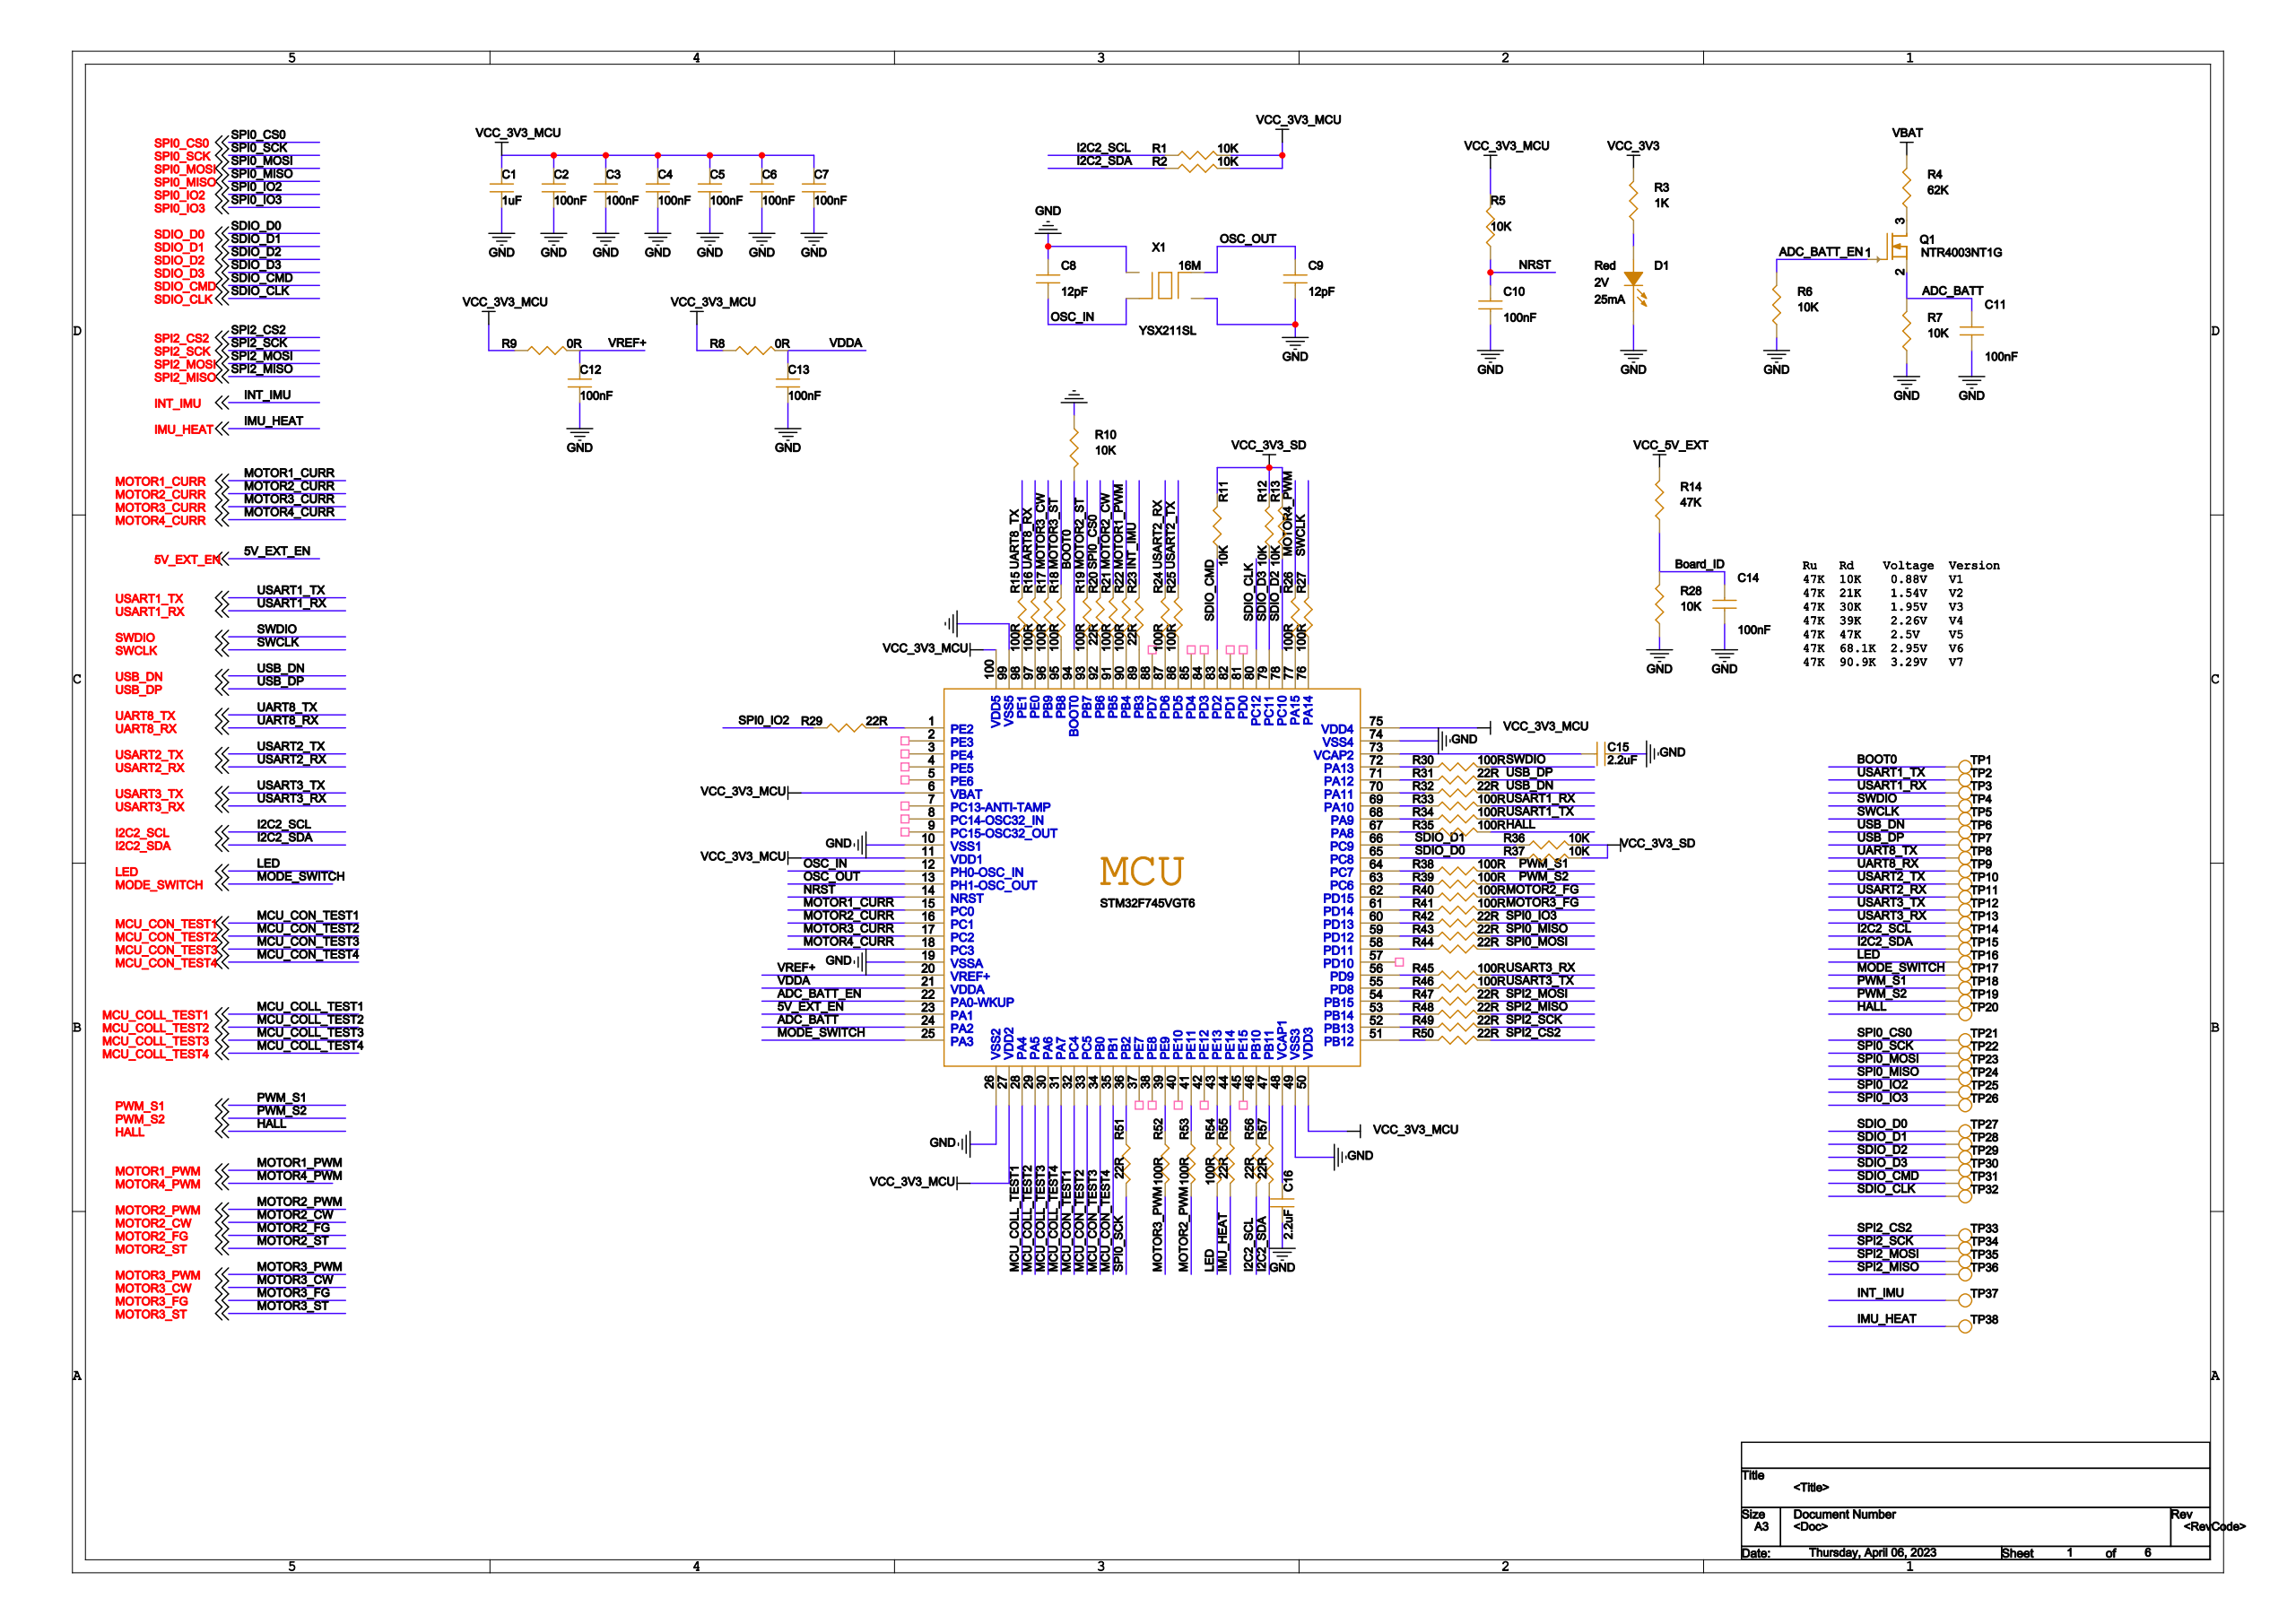Circuit board | Cadence Allegro | 278 parts | 154 nets | one sheet of the schematic
Parts on this sheet (reference | value | footprint):
C1 | 1uF | C0402
C2 | 100nF | C0402
C3 | 100nF | C0402
C4 | 100nF | C0402
C5 | 100nF | C0402
C6 | 100nF | C0402
C7 | 100nF | C0402
C8 | 12pF | C0402
C9 | 12pF | C0402
C10 | 100nF | C0402
C11 | 100nF | C0402
C12 | 100nF | C0402
C13 | 100nF | C0402
C14 | 100nF | C0402
C15 | 2.2uF | C0402
C16 | 2.2uF | C0402
D1 | FC-DA1608HRK-620D | D0603
Q1 | NTR4003NT1G | SOT-23_0
R1 | 10K | R0402
R2 | 10K | R0402
R3 | 1K | R0402
R4 | 62K | R0402
R5 | 10K | R0402
R6 | 10K | R0402
R7 | 10K | R0402
R8 | 0R | R0402
R9 | 0R | R0402
R10 | 10K | R0402
R11 | 10K | R0402
R12 | 10K | R0402
R13 | 10K | R0402
R14 | 47K | R0402
R15 | 100R | R0402
R16 | 100R | R0402
R17 | 100R | R0402
R18 | 100R | R0402
R19 | 100R | R0402
R20 | 22R | R0402
R21 | 100R | R0402
R22 | 100R | R0402
R23 | 22R | R0402
R24 | 100R | R0402
R25 | 100R | R0402
R26 | 100R | R0402
R27 | 100R | R0402
R28 | 10K | R0402
R29 | 22R | R0402
R30 | 100R | R0402
R31 | 22R | R0402
R32 | 22R | R0402
R33 | 100R | R0402
R34 | 100R | R0402
R35 | 100R | R0402
R36 | 10K | R0402
R37 | 10K | R0402
R38 | 100R | R0402
R39 | 100R | R0402
R40 | 100R | R0402
R41 | 100R | R0402
R42 | 22R | R0402
R43 | 22R | R0402
R44 | 22R | R0402
R45 | 100R | R0402
R46 | 100R | R0402
R47 | 22R | R0402
R48 | 22R | R0402
R49 | 22R | R0402
R50 | 22R | R0402
R51 | 22R | R0402
R52 | 100R | R0402
R53 | 100R | R0402
R54 | 100R | R0402
R55 | 22R | R0402
R56 | 22R | R0402
R57 | 22R | R0402
TP1 | T POINT R | TP_C1
TP2 | T POINT R | TP_C1
TP3 | T POINT R | TP_C1
TP4 | T POINT R | TP_C1
TP5 | T POINT R | TP_C1
TP6 | T POINT R | TP_C1
TP7 | T POINT R | TP_C1
TP8 | T POINT R | TP_C1
TP9 | T POINT R | TP_C1
TP10 | T POINT R | TP_C1
TP11 | T POINT R | TP_C1
TP12 | T POINT R | TP_C1
TP13 | T POINT R | TP_C1
TP14 | T POINT R | TP_C1
TP15 | T POINT R | TP_C1
TP16 | T POINT R | TP_C1
TP17 | T POINT R | TP_C1
TP18 | T POINT R | TP_C1
TP19 | T POINT R | TP_C1
TP20 | T POINT R | TP_C1
TP21 | T POINT R | TP_C1
TP22 | T POINT R | TP_C1
TP23 | T POINT R | TP_C1
TP24 | T POINT R | TP_C1
TP25 | T POINT R | TP_C1
TP26 | T POINT R | TP_C1
TP27 | T POINT R | TP_C1
TP28 | T POINT R | TP_C1
TP29 | T POINT R | TP_C1
TP30 | T POINT R | TP_C1
TP31 | T POINT R | TP_C1
TP32 | T POINT R | TP_C1
TP33 | T POINT R | TP_C1
TP34 | T POINT R | TP_C1
TP35 | T POINT R | TP_C1
TP36 | T POINT R | TP_C1
TP37 | T POINT R | TP_C1
TP38 | T POINT R | TP_C1
X1 | YSX211SL | SMD2016
Nets of these parts (net: part-pin ...):
GND: C1-1 C2-1 C3-1 C4-1 C5-1 C6-1 C7-1 C8-1 C9-2 C10-2 C11-1 C12-1 C13-1 C14-1 C15-1 C16-1 D1-1 R6-1 R7-1 R10-1 R28-1 X1-2 X1-4
SDIO_D2: R13-1 TP29-1
USB_DP: R31-2 TP7-1
USB_DN: R32-2 TP6-1
SDIO_D3: R12-1 TP30-1
SDIO_CMD: R11-1 TP31-1
SDIO_CLK: TP32-1
SDIO_D0: R37-1 TP27-1
SDIO_D1: R36-1 TP28-1
OSC_IN: C8-2 X1-1
OSC_OUT: C9-1 X1-3
VCC_3V3_MCU: C1-2 C2-2 C3-2 C4-2 C5-2 C6-2 C7-2 R1-2 R2-2 R5-2 R8-1 R9-1
NRST: C10-1 R5-1
ADC_BATT: C11-2 Q1-2 R7-2
VREF+: C12-2 R9-2
VDDA: C13-2 R8-2
BOARD_ID: C14-2 R14-1 R28-2
VCC_3V3_SD: R11-2 R12-2 R13-2 R36-2 R37-2
VCC_3V3: R3-2
VCC_5V_EXT: R14-2
N16849670: C15-2
N16849769: C16-2
VBAT: R4-2
N16853404: D1-2 R3-1
PWM_S2: R39-2 TP19-1
HALL: R35-2 TP20-1
MOTOR2_PWM: R53-2
MOTOR2_CW: R21-2
MOTOR2_FG: R40-2
MOTOR2_ST: R19-2
MOTOR4_PWM: R26-2
MOTOR3_PWM: R52-2
MOTOR3_CW: R17-2
MOTOR3_FG: R41-2
MOTOR3_ST: R18-2
MOTOR1_PWM: R22-2
PWM_S1: R38-2 TP18-1
I2C2_SCL: R1-1 R56-2 TP14-1
I2C2_SDA: R2-1 R57-2 TP15-1
LED: R54-2 TP16-1
MODE_SWITCH: TP17-1
USART2_TX: R25-2 TP10-1
USART2_RX: R24-2 TP11-1
USART3_TX: R46-2 TP12-1
USART3_RX: R45-2 TP13-1
USART1_TX: R34-2 TP2-1
USART1_RX: R33-2 TP3-1
SWDIO: R30-2 TP4-1
SWCLK: R27-2 TP5-1
UART8_TX: R15-2 TP8-1
UART8_RX: R16-2 TP9-1
N168537470: Q1-3 R4-1
ADC_BATT_EN: Q1-1 R6-2
IMU_HEAT: R55-2 TP38-1
BOOT0: R10-2 TP1-1
N103622976: R15-1
N103622977: R16-1
N103622978: R17-1
N103622979: R18-1
N103622981: R19-1
N103622983: R21-1
N103622984: R22-1
N103622987: R24-1
N103622988: R25-1
N103622997: R26-1
N103622998: R27-1
N16816920: R30-1
N16817350: R33-1
N16817301: R34-1
N16841755: R35-1
N16841714: R38-1
N16841717: R39-1
N16854449: R40-1
N16854452: R41-1
N16820611: R45-1
N16820597: R46-1
N16841155: R52-1
N16841125: R53-1
N16841088: R54-1
N103622982: R20-1
SPI0_CS0: R20-2 TP21-1
N103622985: R23-1
INT_IMU: R23-2 TP37-1
SPI0_IO2: R29-1 TP25-1
N16821071: R29-2
N16819762: R31-1
N16819776: R32-1
N16821115: R42-1
SPI0_IO3: R42-2 TP26-1
N16821043: R43-1
SPI0_MISO: R43-2 TP24-1
N16821000: R44-1
SPI0_MOSI: R44-2 TP23-1
N16821649: R47-1
SPI2_MOSI: R47-2 TP35-1
N16821651: R48-1
SPI2_MISO: R48-2 TP36-1
N16821652: R49-1
SPI2_SCK: R49-2 TP34-1
N16842802: R50-1
SPI2_CS2: R50-2 TP33-1
N16821150: R51-1
SPI0_SCK: R51-2 TP22-1
N16841026: R55-1
N16821381: R56-1
N16843559: R57-1